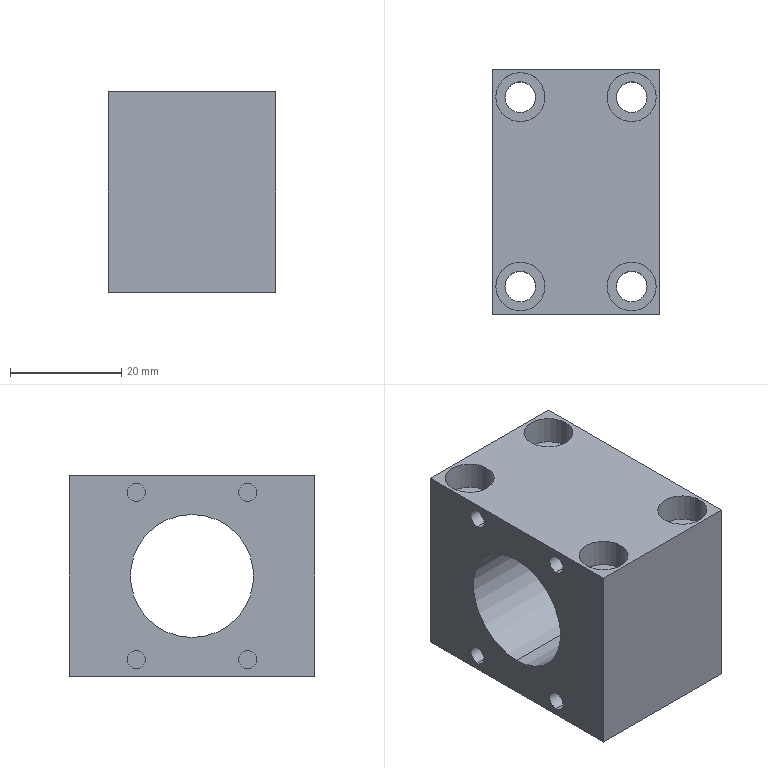Part | SolidWorks | features BaseBody 1 | 1 solid | 52 faces | box 30 x 44 x 36 mm | volume 31000 mm3 | cylinder 34 | plane 18 | commonest cylinder face diameters 3.3 x16 5.5 x8 8.8 x8 22.1 x2
STEP:
#1=CARTESIAN_POINT('',(-15.,0.,29.05));
#2=VERTEX_POINT('',#1);
#3=CARTESIAN_POINT('',(-15.,0.,6.95));
#4=VERTEX_POINT('',#3);
#5=CARTESIAN_POINT('',(-15.,0.,18.));
#6=DIRECTION('',(1.,0.,0.));
#7=DIRECTION('',(0.,0.,-1.));
#8=AXIS2_PLACEMENT_3D('',#5,#6,#7);
#9=CIRCLE('',#8,11.05);
#10=EDGE_CURVE('',#2,#4,#9,.T.);
#11=ORIENTED_EDGE('',*,*,#10,.F.);
#12=CARTESIAN_POINT('',(15.,0.,29.05));
#13=VERTEX_POINT('',#12);
#14=CARTESIAN_POINT('',(-16.,0.,29.05));
#15=DIRECTION('',(1.,0.,0.));
#16=VECTOR('',#15,1000.);
#17=LINE('',#14,#16);
#18=EDGE_CURVE('',#2,#13,#17,.T.);
#19=ORIENTED_EDGE('',*,*,#18,.T.);
#20=CARTESIAN_POINT('',(15.,0.,6.95));
#21=VERTEX_POINT('',#20);
#22=CARTESIAN_POINT('',(15.,0.,18.));
#23=DIRECTION('',(-1.,0.,0.));
#24=DIRECTION('',(0.,0.,-1.));
#25=AXIS2_PLACEMENT_3D('',#22,#23,#24);
#26=CIRCLE('',#25,11.05);
#27=EDGE_CURVE('',#21,#13,#26,.T.);
#28=ORIENTED_EDGE('',*,*,#27,.F.);
#29=CARTESIAN_POINT('',(-16.,0.,6.95));
#30=DIRECTION('',(1.,0.,0.));
#31=VECTOR('',#30,1000.);
#32=LINE('',#29,#31);
#33=EDGE_CURVE('',#4,#21,#32,.T.);
#34=ORIENTED_EDGE('',*,*,#33,.F.);
#35=EDGE_LOOP('',(#11,#19,#28,#34));
#36=FACE_OUTER_BOUND('',#35,.T.);
#37=CARTESIAN_POINT('',(-16.,0.,18.));
#38=DIRECTION('',(1.,0.,0.));
#39=DIRECTION('',(0.,0.,-1.));
#40=AXIS2_PLACEMENT_3D('',#37,#38,#39);
#41=CYLINDRICAL_SURFACE('',#40,11.05);
#42=ADVANCED_FACE('',(#36),#41,.F.);
#43=CARTESIAN_POINT('',(-2.8,-10.,31.35));
#44=VERTEX_POINT('',#43);
#45=CARTESIAN_POINT('',(-2.8,-10.,34.65));
#46=VERTEX_POINT('',#45);
#47=CARTESIAN_POINT('',(-2.8,-10.,33.));
#48=DIRECTION('',(-1.,0.,0.));
#49=DIRECTION('',(0.,0.,1.));
#50=AXIS2_PLACEMENT_3D('',#47,#48,#49);
#51=CIRCLE('',#50,1.65);
#52=EDGE_CURVE('',#44,#46,#51,.T.);
#53=ORIENTED_EDGE('',*,*,#52,.F.);
#54=CARTESIAN_POINT('',(-15.,-10.,31.35));
#55=VERTEX_POINT('',#54);
#56=CARTESIAN_POINT('',(-2.8,-10.,31.35));
#57=DIRECTION('',(-1.,0.,0.));
#58=VECTOR('',#57,1000.);
#59=LINE('',#56,#58);
#60=EDGE_CURVE('',#44,#55,#59,.T.);
#61=ORIENTED_EDGE('',*,*,#60,.T.);
#62=CARTESIAN_POINT('',(-15.,-10.,34.65));
#63=VERTEX_POINT('',#62);
#64=CARTESIAN_POINT('',(-15.,-10.,33.));
#65=DIRECTION('',(-1.,0.,0.));
#66=DIRECTION('',(0.,0.,1.));
#67=AXIS2_PLACEMENT_3D('',#64,#65,#66);
#68=CIRCLE('',#67,1.65);
#69=EDGE_CURVE('',#55,#63,#68,.T.);
#70=ORIENTED_EDGE('',*,*,#69,.T.);
#71=CARTESIAN_POINT('',(-2.8,-10.,34.65));
#72=DIRECTION('',(-1.,0.,0.));
#73=VECTOR('',#72,1000.);
#74=LINE('',#71,#73);
#75=EDGE_CURVE('',#46,#63,#74,.T.);
#76=ORIENTED_EDGE('',*,*,#75,.F.);
#77=EDGE_LOOP('',(#53,#61,#70,#76));
#78=FACE_OUTER_BOUND('',#77,.T.);
#79=CARTESIAN_POINT('',(-2.8,-10.,33.));
#80=DIRECTION('',(-1.,0.,0.));
#81=DIRECTION('',(0.,0.,1.));
#82=AXIS2_PLACEMENT_3D('',#79,#80,#81);
#83=CYLINDRICAL_SURFACE('',#82,1.65);
#84=ADVANCED_FACE('',(#78),#83,.F.);
#85=CARTESIAN_POINT('',(-2.8,-10.,1.35));
#86=VERTEX_POINT('',#85);
#87=CARTESIAN_POINT('',(-2.8,-10.,4.65));
#88=VERTEX_POINT('',#87);
#89=CARTESIAN_POINT('',(-2.8,-10.,3.));
#90=DIRECTION('',(-1.,0.,0.));
#91=DIRECTION('',(0.,0.,1.));
#92=AXIS2_PLACEMENT_3D('',#89,#90,#91);
#93=CIRCLE('',#92,1.65);
#94=EDGE_CURVE('',#86,#88,#93,.T.);
#95=ORIENTED_EDGE('',*,*,#94,.F.);
#96=CARTESIAN_POINT('',(-15.,-10.,1.35));
#97=VERTEX_POINT('',#96);
#98=CARTESIAN_POINT('',(-2.8,-10.,1.35));
#99=DIRECTION('',(-1.,0.,0.));
#100=VECTOR('',#99,1000.);
#101=LINE('',#98,#100);
#102=EDGE_CURVE('',#86,#97,#101,.T.);
#103=ORIENTED_EDGE('',*,*,#102,.T.);
#104=CARTESIAN_POINT('',(-15.,-10.,4.65));
#105=VERTEX_POINT('',#104);
#106=CARTESIAN_POINT('',(-15.,-10.,3.));
#107=DIRECTION('',(-1.,0.,0.));
#108=DIRECTION('',(0.,0.,1.));
#109=AXIS2_PLACEMENT_3D('',#106,#107,#108);
#110=CIRCLE('',#109,1.65);
#111=EDGE_CURVE('',#97,#105,#110,.T.);
#112=ORIENTED_EDGE('',*,*,#111,.T.);
#113=CARTESIAN_POINT('',(-2.8,-10.,4.65));
#114=DIRECTION('',(-1.,0.,0.));
#115=VECTOR('',#114,1000.);
#116=LINE('',#113,#115);
#117=EDGE_CURVE('',#88,#105,#116,.T.);
#118=ORIENTED_EDGE('',*,*,#117,.F.);
#119=EDGE_LOOP('',(#95,#103,#112,#118));
#120=FACE_OUTER_BOUND('',#119,.T.);
#121=CARTESIAN_POINT('',(-2.8,-10.,3.));
#122=DIRECTION('',(-1.,0.,0.));
#123=DIRECTION('',(0.,0.,1.));
#124=AXIS2_PLACEMENT_3D('',#121,#122,#123);
#125=CYLINDRICAL_SURFACE('',#124,1.65);
#126=ADVANCED_FACE('',(#120),#125,.F.);
#127=CARTESIAN_POINT('',(-2.8,10.,31.35));
#128=VERTEX_POINT('',#127);
#129=CARTESIAN_POINT('',(-2.8,10.,34.65));
#130=VERTEX_POINT('',#129);
#131=CARTESIAN_POINT('',(-2.8,10.,33.));
#132=DIRECTION('',(-1.,0.,0.));
#133=DIRECTION('',(0.,0.,1.));
#134=AXIS2_PLACEMENT_3D('',#131,#132,#133);
#135=CIRCLE('',#134,1.65);
#136=EDGE_CURVE('',#128,#130,#135,.T.);
#137=ORIENTED_EDGE('',*,*,#136,.F.);
#138=CARTESIAN_POINT('',(-15.,10.,31.35));
#139=VERTEX_POINT('',#138);
#140=CARTESIAN_POINT('',(-2.8,10.,31.35));
#141=DIRECTION('',(-1.,0.,0.));
#142=VECTOR('',#141,1000.);
#143=LINE('',#140,#142);
#144=EDGE_CURVE('',#128,#139,#143,.T.);
#145=ORIENTED_EDGE('',*,*,#144,.T.);
#146=CARTESIAN_POINT('',(-15.,10.,34.65));
#147=VERTEX_POINT('',#146);
#148=CARTESIAN_POINT('',(-15.,10.,33.));
#149=DIRECTION('',(-1.,0.,0.));
#150=DIRECTION('',(0.,0.,1.));
#151=AXIS2_PLACEMENT_3D('',#148,#149,#150);
#152=CIRCLE('',#151,1.65);
#153=EDGE_CURVE('',#139,#147,#152,.T.);
#154=ORIENTED_EDGE('',*,*,#153,.T.);
#155=CARTESIAN_POINT('',(-2.8,10.,34.65));
#156=DIRECTION('',(-1.,0.,0.));
#157=VECTOR('',#156,1000.);
#158=LINE('',#155,#157);
#159=EDGE_CURVE('',#130,#147,#158,.T.);
#160=ORIENTED_EDGE('',*,*,#159,.F.);
#161=EDGE_LOOP('',(#137,#145,#154,#160));
#162=FACE_OUTER_BOUND('',#161,.T.);
#163=CARTESIAN_POINT('',(-2.8,10.,33.));
#164=DIRECTION('',(-1.,0.,0.));
#165=DIRECTION('',(0.,0.,1.));
#166=AXIS2_PLACEMENT_3D('',#163,#164,#165);
#167=CYLINDRICAL_SURFACE('',#166,1.65);
#168=ADVANCED_FACE('',(#162),#167,.F.);
#169=CARTESIAN_POINT('',(-2.8,10.,1.35));
#170=VERTEX_POINT('',#169);
#171=CARTESIAN_POINT('',(-2.8,10.,4.65));
#172=VERTEX_POINT('',#171);
#173=CARTESIAN_POINT('',(-2.8,10.,3.));
#174=DIRECTION('',(-1.,0.,0.));
#175=DIRECTION('',(0.,0.,1.));
#176=AXIS2_PLACEMENT_3D('',#173,#174,#175);
#177=CIRCLE('',#176,1.65);
#178=EDGE_CURVE('',#170,#172,#177,.T.);
#179=ORIENTED_EDGE('',*,*,#178,.F.);
#180=CARTESIAN_POINT('',(-15.,10.,1.35));
#181=VERTEX_POINT('',#180);
#182=CARTESIAN_POINT('',(-2.8,10.,1.35));
#183=DIRECTION('',(-1.,0.,0.));
#184=VECTOR('',#183,1000.);
#185=LINE('',#182,#184);
#186=EDGE_CURVE('',#170,#181,#185,.T.);
#187=ORIENTED_EDGE('',*,*,#186,.T.);
#188=CARTESIAN_POINT('',(-15.,10.,4.65));
#189=VERTEX_POINT('',#188);
#190=CARTESIAN_POINT('',(-15.,10.,3.));
#191=DIRECTION('',(-1.,0.,0.));
#192=DIRECTION('',(0.,0.,1.));
#193=AXIS2_PLACEMENT_3D('',#190,#191,#192);
#194=CIRCLE('',#193,1.65);
#195=EDGE_CURVE('',#181,#189,#194,.T.);
#196=ORIENTED_EDGE('',*,*,#195,.T.);
#197=CARTESIAN_POINT('',(-2.8,10.,4.65));
#198=DIRECTION('',(-1.,0.,0.));
#199=VECTOR('',#198,1000.);
#200=LINE('',#197,#199);
#201=EDGE_CURVE('',#172,#189,#200,.T.);
#202=ORIENTED_EDGE('',*,*,#201,.F.);
#203=EDGE_LOOP('',(#179,#187,#196,#202));
#204=FACE_OUTER_BOUND('',#203,.T.);
#205=CARTESIAN_POINT('',(-2.8,10.,3.));
#206=DIRECTION('',(-1.,0.,0.));
#207=DIRECTION('',(0.,0.,1.));
#208=AXIS2_PLACEMENT_3D('',#205,#206,#207);
#209=CYLINDRICAL_SURFACE('',#208,1.65);
#210=ADVANCED_FACE('',(#204),#209,.F.);
#211=CARTESIAN_POINT('',(2.8,-10.,34.65));
#212=VERTEX_POINT('',#211);
#213=CARTESIAN_POINT('',(2.8,-10.,31.35));
#214=VERTEX_POINT('',#213);
#215=CARTESIAN_POINT('',(2.8,-10.,33.));
#216=DIRECTION('',(1.,0.,0.));
#217=DIRECTION('',(0.,0.,-1.));
#218=AXIS2_PLACEMENT_3D('',#215,#216,#217);
#219=CIRCLE('',#218,1.65);
#220=EDGE_CURVE('',#212,#214,#219,.T.);
#221=ORIENTED_EDGE('',*,*,#220,.F.);
#222=CARTESIAN_POINT('',(15.,-10.,34.65));
#223=VERTEX_POINT('',#222);
#224=CARTESIAN_POINT('',(2.8,-10.,34.65));
#225=DIRECTION('',(1.,0.,0.));
#226=VECTOR('',#225,1000.);
#227=LINE('',#224,#226);
#228=EDGE_CURVE('',#212,#223,#227,.T.);
#229=ORIENTED_EDGE('',*,*,#228,.T.);
#230=CARTESIAN_POINT('',(15.,-10.,31.35));
#231=VERTEX_POINT('',#230);
#232=CARTESIAN_POINT('',(15.,-10.,33.));
#233=DIRECTION('',(-1.,0.,0.));
#234=DIRECTION('',(0.,0.,-1.));
#235=AXIS2_PLACEMENT_3D('',#232,#233,#234);
#236=CIRCLE('',#235,1.65);
#237=EDGE_CURVE('',#231,#223,#236,.T.);
#238=ORIENTED_EDGE('',*,*,#237,.F.);
#239=CARTESIAN_POINT('',(2.8,-10.,31.35));
#240=DIRECTION('',(1.,0.,0.));
#241=VECTOR('',#240,1000.);
#242=LINE('',#239,#241);
#243=EDGE_CURVE('',#214,#231,#242,.T.);
#244=ORIENTED_EDGE('',*,*,#243,.F.);
#245=EDGE_LOOP('',(#221,#229,#238,#244));
#246=FACE_OUTER_BOUND('',#245,.T.);
#247=CARTESIAN_POINT('',(2.8,-10.,33.));
#248=DIRECTION('',(1.,0.,0.));
#249=DIRECTION('',(0.,0.,-1.));
#250=AXIS2_PLACEMENT_3D('',#247,#248,#249);
#251=CYLINDRICAL_SURFACE('',#250,1.65);
#252=ADVANCED_FACE('',(#246),#251,.F.);
#253=CARTESIAN_POINT('',(2.8,-10.,4.65));
#254=VERTEX_POINT('',#253);
#255=CARTESIAN_POINT('',(2.8,-10.,1.35));
#256=VERTEX_POINT('',#255);
#257=CARTESIAN_POINT('',(2.8,-10.,3.));
#258=DIRECTION('',(1.,0.,0.));
#259=DIRECTION('',(0.,0.,-1.));
#260=AXIS2_PLACEMENT_3D('',#257,#258,#259);
#261=CIRCLE('',#260,1.65);
#262=EDGE_CURVE('',#254,#256,#261,.T.);
#263=ORIENTED_EDGE('',*,*,#262,.F.);
#264=CARTESIAN_POINT('',(15.,-10.,4.65));
#265=VERTEX_POINT('',#264);
#266=CARTESIAN_POINT('',(2.8,-10.,4.65));
#267=DIRECTION('',(1.,0.,0.));
#268=VECTOR('',#267,1000.);
#269=LINE('',#266,#268);
#270=EDGE_CURVE('',#254,#265,#269,.T.);
#271=ORIENTED_EDGE('',*,*,#270,.T.);
#272=CARTESIAN_POINT('',(15.,-10.,1.35));
#273=VERTEX_POINT('',#272);
#274=CARTESIAN_POINT('',(15.,-10.,3.));
#275=DIRECTION('',(-1.,0.,0.));
#276=DIRECTION('',(0.,0.,-1.));
#277=AXIS2_PLACEMENT_3D('',#274,#275,#276);
#278=CIRCLE('',#277,1.65);
#279=EDGE_CURVE('',#273,#265,#278,.T.);
#280=ORIENTED_EDGE('',*,*,#279,.F.);
#281=CARTESIAN_POINT('',(2.8,-10.,1.35));
#282=DIRECTION('',(1.,0.,0.));
#283=VECTOR('',#282,1000.);
#284=LINE('',#281,#283);
#285=EDGE_CURVE('',#256,#273,#284,.T.);
#286=ORIENTED_EDGE('',*,*,#285,.F.);
#287=EDGE_LOOP('',(#263,#271,#280,#286));
#288=FACE_OUTER_BOUND('',#287,.T.);
#289=CARTESIAN_POINT('',(2.8,-10.,3.));
#290=DIRECTION('',(1.,0.,0.));
#291=DIRECTION('',(0.,0.,-1.));
#292=AXIS2_PLACEMENT_3D('',#289,#290,#291);
#293=CYLINDRICAL_SURFACE('',#292,1.65);
#294=ADVANCED_FACE('',(#288),#293,.F.);
#295=CARTESIAN_POINT('',(2.8,10.,34.65));
#296=VERTEX_POINT('',#295);
#297=CARTESIAN_POINT('',(2.8,10.,31.35));
#298=VERTEX_POINT('',#297);
#299=CARTESIAN_POINT('',(2.8,10.,33.));
#300=DIRECTION('',(1.,0.,0.));
#301=DIRECTION('',(0.,0.,-1.));
#302=AXIS2_PLACEMENT_3D('',#299,#300,#301);
#303=CIRCLE('',#302,1.65);
#304=EDGE_CURVE('',#296,#298,#303,.T.);
#305=ORIENTED_EDGE('',*,*,#304,.F.);
#306=CARTESIAN_POINT('',(15.,10.,34.65));
#307=VERTEX_POINT('',#306);
#308=CARTESIAN_POINT('',(2.8,10.,34.65));
#309=DIRECTION('',(1.,0.,0.));
#310=VECTOR('',#309,1000.);
#311=LINE('',#308,#310);
#312=EDGE_CURVE('',#296,#307,#311,.T.);
#313=ORIENTED_EDGE('',*,*,#312,.T.);
#314=CARTESIAN_POINT('',(15.,10.,31.35));
#315=VERTEX_POINT('',#314);
#316=CARTESIAN_POINT('',(15.,10.,33.));
#317=DIRECTION('',(-1.,0.,0.));
#318=DIRECTION('',(0.,0.,-1.));
#319=AXIS2_PLACEMENT_3D('',#316,#317,#318);
#320=CIRCLE('',#319,1.65);
#321=EDGE_CURVE('',#315,#307,#320,.T.);
#322=ORIENTED_EDGE('',*,*,#321,.F.);
#323=CARTESIAN_POINT('',(2.8,10.,31.35));
#324=DIRECTION('',(1.,0.,0.));
#325=VECTOR('',#324,1000.);
#326=LINE('',#323,#325);
#327=EDGE_CURVE('',#298,#315,#326,.T.);
#328=ORIENTED_EDGE('',*,*,#327,.F.);
#329=EDGE_LOOP('',(#305,#313,#322,#328));
#330=FACE_OUTER_BOUND('',#329,.T.);
#331=CARTESIAN_POINT('',(2.8,10.,33.));
#332=DIRECTION('',(1.,0.,0.));
#333=DIRECTION('',(0.,0.,-1.));
#334=AXIS2_PLACEMENT_3D('',#331,#332,#333);
#335=CYLINDRICAL_SURFACE('',#334,1.65);
#336=ADVANCED_FACE('',(#330),#335,.F.);
#337=CARTESIAN_POINT('',(2.8,10.,4.65));
#338=VERTEX_POINT('',#337);
#339=CARTESIAN_POINT('',(2.8,10.,1.35));
#340=VERTEX_POINT('',#339);
#341=CARTESIAN_POINT('',(2.8,10.,3.));
#342=DIRECTION('',(1.,0.,0.));
#343=DIRECTION('',(0.,0.,-1.));
#344=AXIS2_PLACEMENT_3D('',#341,#342,#343);
#345=CIRCLE('',#344,1.65);
#346=EDGE_CURVE('',#338,#340,#345,.T.);
#347=ORIENTED_EDGE('',*,*,#346,.F.);
#348=CARTESIAN_POINT('',(15.,10.,4.65));
#349=VERTEX_POINT('',#348);
#350=CARTESIAN_POINT('',(2.8,10.,4.65));
#351=DIRECTION('',(1.,0.,0.));
#352=VECTOR('',#351,1000.);
#353=LINE('',#350,#352);
#354=EDGE_CURVE('',#338,#349,#353,.T.);
#355=ORIENTED_EDGE('',*,*,#354,.T.);
#356=CARTESIAN_POINT('',(15.,10.,1.35));
#357=VERTEX_POINT('',#356);
#358=CARTESIAN_POINT('',(15.,10.,3.));
#359=DIRECTION('',(-1.,0.,0.));
#360=DIRECTION('',(0.,0.,-1.));
#361=AXIS2_PLACEMENT_3D('',#358,#359,#360);
#362=CIRCLE('',#361,1.65);
#363=EDGE_CURVE('',#357,#349,#362,.T.);
#364=ORIENTED_EDGE('',*,*,#363,.F.);
#365=CARTESIAN_POINT('',(2.8,10.,1.35));
#366=DIRECTION('',(1.,0.,0.));
#367=VECTOR('',#366,1000.);
#368=LINE('',#365,#367);
#369=EDGE_CURVE('',#340,#357,#368,.T.);
#370=ORIENTED_EDGE('',*,*,#369,.F.);
#371=EDGE_LOOP('',(#347,#355,#364,#370));
#372=FACE_OUTER_BOUND('',#371,.T.);
#373=CARTESIAN_POINT('',(2.8,10.,3.));
#374=DIRECTION('',(1.,0.,0.));
#375=DIRECTION('',(0.,0.,-1.));
#376=AXIS2_PLACEMENT_3D('',#373,#374,#375);
#377=CYLINDRICAL_SURFACE('',#376,1.65);
#378=ADVANCED_FACE('',(#372),#377,.F.);
#379=CARTESIAN_POINT('',(5.6,17.,30.9));
#380=VERTEX_POINT('',#379);
#381=CARTESIAN_POINT('',(14.4,17.,30.9));
#382=VERTEX_POINT('',#381);
#383=CARTESIAN_POINT('',(10.,17.,30.9));
#384=DIRECTION('',(0.,0.,1.));
#385=DIRECTION('',(1.,0.,0.));
#386=AXIS2_PLACEMENT_3D('',#383,#384,#385);
#387=CIRCLE('',#386,4.4);
#388=EDGE_CURVE('',#380,#382,#387,.T.);
#389=ORIENTED_EDGE('',*,*,#388,.F.);
#390=CARTESIAN_POINT('',(5.6,17.,36.));
#391=VERTEX_POINT('',#390);
#392=CARTESIAN_POINT('',(5.6,17.,30.9));
#393=DIRECTION('',(0.,0.,1.));
#394=VECTOR('',#393,1000.);
#395=LINE('',#392,#394);
#396=EDGE_CURVE('',#380,#391,#395,.T.);
#397=ORIENTED_EDGE('',*,*,#396,.T.);
#398=CARTESIAN_POINT('',(14.4,17.,36.));
#399=VERTEX_POINT('',#398);
#400=CARTESIAN_POINT('',(10.,17.,36.));
#401=DIRECTION('',(0.,0.,-1.));
#402=DIRECTION('',(1.,0.,0.));
#403=AXIS2_PLACEMENT_3D('',#400,#401,#402);
#404=CIRCLE('',#403,4.4);
#405=EDGE_CURVE('',#399,#391,#404,.T.);
#406=ORIENTED_EDGE('',*,*,#405,.F.);
#407=CARTESIAN_POINT('',(14.4,17.,30.9));
#408=DIRECTION('',(0.,0.,1.));
#409=VECTOR('',#408,1000.);
#410=LINE('',#407,#409);
#411=EDGE_CURVE('',#382,#399,#410,.T.);
#412=ORIENTED_EDGE('',*,*,#411,.F.);
#413=EDGE_LOOP('',(#389,#397,#406,#412));
#414=FACE_OUTER_BOUND('',#413,.T.);
#415=CARTESIAN_POINT('',(10.,17.,30.9));
#416=DIRECTION('',(0.,0.,1.));
#417=DIRECTION('',(1.,0.,0.));
#418=AXIS2_PLACEMENT_3D('',#415,#416,#417);
#419=CYLINDRICAL_SURFACE('',#418,4.4);
#420=ADVANCED_FACE('',(#414),#419,.F.);
#421=CARTESIAN_POINT('',(-14.4,17.,30.9));
#422=VERTEX_POINT('',#421);
#423=CARTESIAN_POINT('',(-5.6,17.,30.9));
#424=VERTEX_POINT('',#423);
#425=CARTESIAN_POINT('',(-10.,17.,30.9));
#426=DIRECTION('',(0.,0.,1.));
#427=DIRECTION('',(1.,0.,0.));
#428=AXIS2_PLACEMENT_3D('',#425,#426,#427);
#429=CIRCLE('',#428,4.4);
#430=EDGE_CURVE('',#422,#424,#429,.T.);
#431=ORIENTED_EDGE('',*,*,#430,.F.);
#432=CARTESIAN_POINT('',(-14.4,17.,36.));
#433=VERTEX_POINT('',#432);
#434=CARTESIAN_POINT('',(-14.4,17.,30.9));
#435=DIRECTION('',(0.,0.,1.));
#436=VECTOR('',#435,1000.);
#437=LINE('',#434,#436);
#438=EDGE_CURVE('',#422,#433,#437,.T.);
#439=ORIENTED_EDGE('',*,*,#438,.T.);
#440=CARTESIAN_POINT('',(-5.6,17.,36.));
#441=VERTEX_POINT('',#440);
#442=CARTESIAN_POINT('',(-10.,17.,36.));
#443=DIRECTION('',(0.,0.,-1.));
#444=DIRECTION('',(1.,0.,0.));
#445=AXIS2_PLACEMENT_3D('',#442,#443,#444);
#446=CIRCLE('',#445,4.4);
#447=EDGE_CURVE('',#441,#433,#446,.T.);
#448=ORIENTED_EDGE('',*,*,#447,.F.);
#449=CARTESIAN_POINT('',(-5.6,17.,30.9));
#450=DIRECTION('',(0.,0.,1.));
#451=VECTOR('',#450,1000.);
#452=LINE('',#449,#451);
#453=EDGE_CURVE('',#424,#441,#452,.T.);
#454=ORIENTED_EDGE('',*,*,#453,.F.);
#455=EDGE_LOOP('',(#431,#439,#448,#454));
#456=FACE_OUTER_BOUND('',#455,.T.);
#457=CARTESIAN_POINT('',(-10.,17.,30.9));
#458=DIRECTION('',(0.,0.,1.));
#459=DIRECTION('',(1.,0.,0.));
#460=AXIS2_PLACEMENT_3D('',#457,#458,#459);
#461=CYLINDRICAL_SURFACE('',#460,4.4);
#462=ADVANCED_FACE('',(#456),#461,.F.);
#463=CARTESIAN_POINT('',(5.6,-17.,30.9));
#464=VERTEX_POINT('',#463);
#465=CARTESIAN_POINT('',(14.4,-17.,30.9));
#466=VERTEX_POINT('',#465);
#467=CARTESIAN_POINT('',(10.,-17.,30.9));
#468=DIRECTION('',(0.,0.,1.));
#469=DIRECTION('',(1.,0.,0.));
#470=AXIS2_PLACEMENT_3D('',#467,#468,#469);
#471=CIRCLE('',#470,4.4);
#472=EDGE_CURVE('',#464,#466,#471,.T.);
#473=ORIENTED_EDGE('',*,*,#472,.F.);
#474=CARTESIAN_POINT('',(5.6,-17.,36.));
#475=VERTEX_POINT('',#474);
#476=CARTESIAN_POINT('',(5.6,-17.,30.9));
#477=DIRECTION('',(0.,0.,1.));
#478=VECTOR('',#477,1000.);
#479=LINE('',#476,#478);
#480=EDGE_CURVE('',#464,#475,#479,.T.);
#481=ORIENTED_EDGE('',*,*,#480,.T.);
#482=CARTESIAN_POINT('',(14.4,-17.,36.));
#483=VERTEX_POINT('',#482);
#484=CARTESIAN_POINT('',(10.,-17.,36.));
#485=DIRECTION('',(0.,0.,-1.));
#486=DIRECTION('',(1.,0.,0.));
#487=AXIS2_PLACEMENT_3D('',#484,#485,#486);
#488=CIRCLE('',#487,4.4);
#489=EDGE_CURVE('',#483,#475,#488,.T.);
#490=ORIENTED_EDGE('',*,*,#489,.F.);
#491=CARTESIAN_POINT('',(14.4,-17.,30.9));
#492=DIRECTION('',(0.,0.,1.));
#493=VECTOR('',#492,1000.);
#494=LINE('',#491,#493);
#495=EDGE_CURVE('',#466,#483,#494,.T.);
#496=ORIENTED_EDGE('',*,*,#495,.F.);
#497=EDGE_LOOP('',(#473,#481,#490,#496));
#498=FACE_OUTER_BOUND('',#497,.T.);
#499=CARTESIAN_POINT('',(10.,-17.,30.9));
#500=DIRECTION('',(0.,0.,1.));
#501=DIRECTION('',(1.,0.,0.));
#502=AXIS2_PLACEMENT_3D('',#499,#500,#501);
#503=CYLINDRICAL_SURFACE('',#502,4.4);
#504=ADVANCED_FACE('',(#498),#503,.F.);
#505=CARTESIAN_POINT('',(-14.4,-17.,30.9));
#506=VERTEX_POINT('',#505);
#507=CARTESIAN_POINT('',(-5.6,-17.,30.9));
#508=VERTEX_POINT('',#507);
#509=CARTESIAN_POINT('',(-10.,-17.,30.9));
#510=DIRECTION('',(0.,0.,1.));
#511=DIRECTION('',(1.,0.,0.));
#512=AXIS2_PLACEMENT_3D('',#509,#510,#511);
#513=CIRCLE('',#512,4.4);
#514=EDGE_CURVE('',#506,#508,#513,.T.);
#515=ORIENTED_EDGE('',*,*,#514,.F.);
#516=CARTESIAN_POINT('',(-14.4,-17.,36.));
#517=VERTEX_POINT('',#516);
#518=CARTESIAN_POINT('',(-14.4,-17.,30.9));
#519=DIRECTION('',(0.,0.,1.));
#520=VECTOR('',#519,1000.);
#521=LINE('',#518,#520);
#522=EDGE_CURVE('',#506,#517,#521,.T.);
#523=ORIENTED_EDGE('',*,*,#522,.T.);
#524=CARTESIAN_POINT('',(-5.6,-17.,36.));
#525=VERTEX_POINT('',#524);
#526=CARTESIAN_POINT('',(-10.,-17.,36.));
#527=DIRECTION('',(0.,0.,-1.));
#528=DIRECTION('',(1.,0.,0.));
#529=AXIS2_PLACEMENT_3D('',#526,#527,#528);
#530=CIRCLE('',#529,4.4);
#531=EDGE_CURVE('',#525,#517,#530,.T.);
#532=ORIENTED_EDGE('',*,*,#531,.F.);
#533=CARTESIAN_POINT('',(-5.6,-17.,30.9));
#534=DIRECTION('',(0.,0.,1.));
#535=VECTOR('',#534,1000.);
#536=LINE('',#533,#535);
#537=EDGE_CURVE('',#508,#525,#536,.T.);
#538=ORIENTED_EDGE('',*,*,#537,.F.);
#539=EDGE_LOOP('',(#515,#523,#532,#538));
#540=FACE_OUTER_BOUND('',#539,.T.);
#541=CARTESIAN_POINT('',(-10.,-17.,30.9));
#542=DIRECTION('',(0.,0.,1.));
#543=DIRECTION('',(1.,0.,0.));
#544=AXIS2_PLACEMENT_3D('',#541,#542,#543);
#545=CYLINDRICAL_SURFACE('',#544,4.4);
#546=ADVANCED_FACE('',(#540),#545,.F.);
#547=CARTESIAN_POINT('',(12.75,17.,0.));
#548=VERTEX_POINT('',#547);
#549=CARTESIAN_POINT('',(7.25,17.,0.));
#550=VERTEX_POINT('',#549);
#551=CARTESIAN_POINT('',(10.,17.,0.));
#552=DIRECTION('',(0.,0.,-1.));
#553=DIRECTION('',(1.,0.,0.));
#554=AXIS2_PLACEMENT_3D('',#551,#552,#553);
#555=CIRCLE('',#554,2.75);
#556=EDGE_CURVE('',#548,#550,#555,.T.);
#557=ORIENTED_EDGE('',*,*,#556,.T.);
#558=CARTESIAN_POINT('',(7.25,17.,30.9));
#559=VERTEX_POINT('',#558);
#560=CARTESIAN_POINT('',(7.25,17.,-1.));
#561=DIRECTION('',(0.,0.,1.));
#562=VECTOR('',#561,1000.);
#563=LINE('',#560,#562);
#564=EDGE_CURVE('',#550,#559,#563,.T.);
#565=ORIENTED_EDGE('',*,*,#564,.T.);
#566=CARTESIAN_POINT('',(12.75,17.,30.9));
#567=VERTEX_POINT('',#566);
#568=CARTESIAN_POINT('',(10.,17.,30.9));
#569=DIRECTION('',(0.,0.,-1.));
#570=DIRECTION('',(1.,0.,0.));
#571=AXIS2_PLACEMENT_3D('',#568,#569,#570);
#572=CIRCLE('',#571,2.75);
#573=EDGE_CURVE('',#567,#559,#572,.T.);
#574=ORIENTED_EDGE('',*,*,#573,.F.);
#575=CARTESIAN_POINT('',(12.75,17.,-1.));
#576=DIRECTION('',(0.,0.,1.));
#577=VECTOR('',#576,1000.);
#578=LINE('',#575,#577);
#579=EDGE_CURVE('',#548,#567,#578,.T.);
#580=ORIENTED_EDGE('',*,*,#579,.F.);
#581=EDGE_LOOP('',(#557,#565,#574,#580));
#582=FACE_OUTER_BOUND('',#581,.T.);
#583=CARTESIAN_POINT('',(10.,17.,-1.));
#584=DIRECTION('',(0.,0.,1.));
#585=DIRECTION('',(1.,0.,0.));
#586=AXIS2_PLACEMENT_3D('',#583,#584,#585);
#587=CYLINDRICAL_SURFACE('',#586,2.75);
#588=ADVANCED_FACE('',(#582),#587,.F.);
#589=CARTESIAN_POINT('',(-7.25,17.,0.));
#590=VERTEX_POINT('',#589);
#591=CARTESIAN_POINT('',(-12.75,17.,0.));
#592=VERTEX_POINT('',#591);
#593=CARTESIAN_POINT('',(-10.,17.,0.));
#594=DIRECTION('',(0.,0.,-1.));
#595=DIRECTION('',(1.,0.,0.));
#596=AXIS2_PLACEMENT_3D('',#593,#594,#595);
#597=CIRCLE('',#596,2.75);
#598=EDGE_CURVE('',#590,#592,#597,.T.);
#599=ORIENTED_EDGE('',*,*,#598,.T.);
#600=CARTESIAN_POINT('',(-12.75,17.,30.9));
#601=VERTEX_POINT('',#600);
#602=CARTESIAN_POINT('',(-12.75,17.,-1.));
#603=DIRECTION('',(0.,0.,1.));
#604=VECTOR('',#603,1000.);
#605=LINE('',#602,#604);
#606=EDGE_CURVE('',#592,#601,#605,.T.);
#607=ORIENTED_EDGE('',*,*,#606,.T.);
#608=CARTESIAN_POINT('',(-7.25,17.,30.9));
#609=VERTEX_POINT('',#608);
#610=CARTESIAN_POINT('',(-10.,17.,30.9));
#611=DIRECTION('',(0.,0.,-1.));
#612=DIRECTION('',(1.,0.,0.));
#613=AXIS2_PLACEMENT_3D('',#610,#611,#612);
#614=CIRCLE('',#613,2.75);
#615=EDGE_CURVE('',#609,#601,#614,.T.);
#616=ORIENTED_EDGE('',*,*,#615,.F.);
#617=CARTESIAN_POINT('',(-7.25,17.,-1.));
#618=DIRECTION('',(0.,0.,1.));
#619=VECTOR('',#618,1000.);
#620=LINE('',#617,#619);
#621=EDGE_CURVE('',#590,#609,#620,.T.);
#622=ORIENTED_EDGE('',*,*,#621,.F.);
#623=EDGE_LOOP('',(#599,#607,#616,#622));
#624=FACE_OUTER_BOUND('',#623,.T.);
#625=CARTESIAN_POINT('',(-10.,17.,-1.));
#626=DIRECTION('',(0.,0.,1.));
#627=DIRECTION('',(1.,0.,0.));
#628=AXIS2_PLACEMENT_3D('',#625,#626,#627);
#629=CYLINDRICAL_SURFACE('',#628,2.75);
#630=ADVANCED_FACE('',(#624),#629,.F.);
#631=CARTESIAN_POINT('',(12.75,-17.,0.));
#632=VERTEX_POINT('',#631);
#633=CARTESIAN_POINT('',(7.25,-17.,0.));
#634=VERTEX_POINT('',#633);
#635=CARTESIAN_POINT('',(10.,-17.,0.));
#636=DIRECTION('',(0.,0.,-1.));
#637=DIRECTION('',(1.,0.,0.));
#638=AXIS2_PLACEMENT_3D('',#635,#636,#637);
#639=CIRCLE('',#638,2.75);
#640=EDGE_CURVE('',#632,#634,#639,.T.);
#641=ORIENTED_EDGE('',*,*,#640,.T.);
#642=CARTESIAN_POINT('',(7.25,-17.,30.9));
#643=VERTEX_POINT('',#642);
#644=CARTESIAN_POINT('',(7.25,-17.,-1.));
#645=DIRECTION('',(0.,0.,1.));
#646=VECTOR('',#645,1000.);
#647=LINE('',#644,#646);
#648=EDGE_CURVE('',#634,#643,#647,.T.);
#649=ORIENTED_EDGE('',*,*,#648,.T.);
#650=CARTESIAN_POINT('',(12.75,-17.,30.9));
#651=VERTEX_POINT('',#650);
#652=CARTESIAN_POINT('',(10.,-17.,30.9));
#653=DIRECTION('',(0.,0.,-1.));
#654=DIRECTION('',(1.,0.,0.));
#655=AXIS2_PLACEMENT_3D('',#652,#653,#654);
#656=CIRCLE('',#655,2.75);
#657=EDGE_CURVE('',#651,#643,#656,.T.);
#658=ORIENTED_EDGE('',*,*,#657,.F.);
#659=CARTESIAN_POINT('',(12.75,-17.,-1.));
#660=DIRECTION('',(0.,0.,1.));
#661=VECTOR('',#660,1000.);
#662=LINE('',#659,#661);
#663=EDGE_CURVE('',#632,#651,#662,.T.);
#664=ORIENTED_EDGE('',*,*,#663,.F.);
#665=EDGE_LOOP('',(#641,#649,#658,#664));
#666=FACE_OUTER_BOUND('',#665,.T.);
#667=CARTESIAN_POINT('',(10.,-17.,-1.));
#668=DIRECTION('',(0.,0.,1.));
#669=DIRECTION('',(1.,0.,0.));
#670=AXIS2_PLACEMENT_3D('',#667,#668,#669);
#671=CYLINDRICAL_SURFACE('',#670,2.75);
#672=ADVANCED_FACE('',(#666),#671,.F.);
#673=CARTESIAN_POINT('',(-7.25,-17.,0.));
#674=VERTEX_POINT('',#673);
#675=CARTESIAN_POINT('',(-12.75,-17.,0.));
#676=VERTEX_POINT('',#675);
#677=CARTESIAN_POINT('',(-10.,-17.,0.));
#678=DIRECTION('',(0.,0.,-1.));
#679=DIRECTION('',(1.,0.,0.));
#680=AXIS2_PLACEMENT_3D('',#677,#678,#679);
#681=CIRCLE('',#680,2.75);
#682=EDGE_CURVE('',#674,#676,#681,.T.);
#683=ORIENTED_EDGE('',*,*,#682,.T.);
#684=CARTESIAN_POINT('',(-12.75,-17.,30.9));
#685=VERTEX_POINT('',#684);
#686=CARTESIAN_POINT('',(-12.75,-17.,-1.));
#687=DIRECTION('',(0.,0.,1.));
#688=VECTOR('',#687,1000.);
#689=LINE('',#686,#688);
#690=EDGE_CURVE('',#676,#685,#689,.T.);
#691=ORIENTED_EDGE('',*,*,#690,.T.);
#692=CARTESIAN_POINT('',(-7.25,-17.,30.9));
#693=VERTEX_POINT('',#692);
#694=CARTESIAN_POINT('',(-10.,-17.,30.9));
#695=DIRECTION('',(0.,0.,-1.));
#696=DIRECTION('',(1.,0.,0.));
#697=AXIS2_PLACEMENT_3D('',#694,#695,#696);
#698=CIRCLE('',#697,2.75);
#699=EDGE_CURVE('',#693,#685,#698,.T.);
#700=ORIENTED_EDGE('',*,*,#699,.F.);
#701=CARTESIAN_POINT('',(-7.25,-17.,-1.));
#702=DIRECTION('',(0.,0.,1.));
#703=VECTOR('',#702,1000.);
#704=LINE('',#701,#703);
#705=EDGE_CURVE('',#674,#693,#704,.T.);
#706=ORIENTED_EDGE('',*,*,#705,.F.);
#707=EDGE_LOOP('',(#683,#691,#700,#706));
#708=FACE_OUTER_BOUND('',#707,.T.);
#709=CARTESIAN_POINT('',(-10.,-17.,-1.));
#710=DIRECTION('',(0.,0.,1.));
#711=DIRECTION('',(1.,0.,0.));
#712=AXIS2_PLACEMENT_3D('',#709,#710,#711);
#713=CYLINDRICAL_SURFACE('',#712,2.75);
#714=ADVANCED_FACE('',(#708),#713,.F.);
#715=ORIENTED_EDGE('',*,*,#18,.F.);
#716=CARTESIAN_POINT('',(-15.,0.,18.));
#717=DIRECTION('',(1.,0.,0.));
#718=DIRECTION('',(0.,0.,-1.));
#719=AXIS2_PLACEMENT_3D('',#716,#717,#718);
#720=CIRCLE('',#719,11.05);
#721=EDGE_CURVE('',#4,#2,#720,.T.);
#722=ORIENTED_EDGE('',*,*,#721,.F.);
#723=ORIENTED_EDGE('',*,*,#33,.T.);
#724=CARTESIAN_POINT('',(15.,0.,18.));
#725=DIRECTION('',(-1.,0.,0.));
#726=DIRECTION('',(0.,0.,-1.));
#727=AXIS2_PLACEMENT_3D('',#724,#725,#726);
#728=CIRCLE('',#727,11.05);
#729=EDGE_CURVE('',#13,#21,#728,.T.);
#730=ORIENTED_EDGE('',*,*,#729,.F.);
#731=EDGE_LOOP('',(#715,#722,#723,#730));
#732=FACE_OUTER_BOUND('',#731,.T.);
#733=CARTESIAN_POINT('',(-16.,0.,18.));
#734=DIRECTION('',(1.,0.,0.));
#735=DIRECTION('',(0.,0.,-1.));
#736=AXIS2_PLACEMENT_3D('',#733,#734,#735);
#737=CYLINDRICAL_SURFACE('',#736,11.05);
#738=ADVANCED_FACE('',(#732),#737,.F.);
#739=CARTESIAN_POINT('',(-15.,-10.,33.));
#740=DIRECTION('',(-1.,0.,0.));
#741=DIRECTION('',(0.,0.,1.));
#742=AXIS2_PLACEMENT_3D('',#739,#740,#741);
#743=CIRCLE('',#742,1.65);
#744=EDGE_CURVE('',#63,#55,#743,.T.);
#745=ORIENTED_EDGE('',*,*,#744,.F.);
#746=ORIENTED_EDGE('',*,*,#69,.F.);
#747=EDGE_LOOP('',(#745,#746));
#748=FACE_BOUND('',#747,.T.);
#749=ORIENTED_EDGE('',*,*,#721,.T.);
#750=ORIENTED_EDGE('',*,*,#10,.T.);
#751=EDGE_LOOP('',(#749,#750));
#752=FACE_BOUND('',#751,.T.);
#753=CARTESIAN_POINT('',(-15.,-10.,3.));
#754=DIRECTION('',(-1.,0.,0.));
#755=DIRECTION('',(0.,0.,1.));
#756=AXIS2_PLACEMENT_3D('',#753,#754,#755);
#757=CIRCLE('',#756,1.65);
#758=EDGE_CURVE('',#105,#97,#757,.T.);
#759=ORIENTED_EDGE('',*,*,#758,.F.);
#760=ORIENTED_EDGE('',*,*,#111,.F.);
#761=EDGE_LOOP('',(#759,#760));
#762=FACE_BOUND('',#761,.T.);
#763=CARTESIAN_POINT('',(-15.,10.,33.));
#764=DIRECTION('',(-1.,0.,0.));
#765=DIRECTION('',(0.,0.,1.));
#766=AXIS2_PLACEMENT_3D('',#763,#764,#765);
#767=CIRCLE('',#766,1.65);
#768=EDGE_CURVE('',#147,#139,#767,.T.);
#769=ORIENTED_EDGE('',*,*,#768,.F.);
#770=ORIENTED_EDGE('',*,*,#153,.F.);
#771=EDGE_LOOP('',(#769,#770));
#772=FACE_BOUND('',#771,.T.);
#773=CARTESIAN_POINT('',(-15.,10.,3.));
#774=DIRECTION('',(-1.,0.,0.));
#775=DIRECTION('',(0.,0.,1.));
#776=AXIS2_PLACEMENT_3D('',#773,#774,#775);
#777=CIRCLE('',#776,1.65);
#778=EDGE_CURVE('',#189,#181,#777,.T.);
#779=ORIENTED_EDGE('',*,*,#778,.F.);
#780=ORIENTED_EDGE('',*,*,#195,.F.);
#781=EDGE_LOOP('',(#779,#780));
#782=FACE_BOUND('',#781,.T.);
#783=CARTESIAN_POINT('',(-15.,22.,0.));
#784=VERTEX_POINT('',#783);
#785=CARTESIAN_POINT('',(-15.,22.,36.));
#786=VERTEX_POINT('',#785);
#787=CARTESIAN_POINT('',(-15.,22.,0.));
#788=DIRECTION('',(0.,0.,1.));
#789=VECTOR('',#788,1000.);
#790=LINE('',#787,#789);
#791=EDGE_CURVE('',#784,#786,#790,.T.);
#792=ORIENTED_EDGE('',*,*,#791,.F.);
#793=CARTESIAN_POINT('',(-15.,-22.,0.));
#794=VERTEX_POINT('',#793);
#795=CARTESIAN_POINT('',(-15.,-22.,0.));
#796=DIRECTION('',(0.,1.,0.));
#797=VECTOR('',#796,1000.);
#798=LINE('',#795,#797);
#799=EDGE_CURVE('',#794,#784,#798,.T.);
#800=ORIENTED_EDGE('',*,*,#799,.F.);
#801=CARTESIAN_POINT('',(-15.,-22.,36.));
#802=VERTEX_POINT('',#801);
#803=CARTESIAN_POINT('',(-15.,-22.,0.));
#804=DIRECTION('',(0.,0.,-1.));
#805=VECTOR('',#804,1000.);
#806=LINE('',#803,#805);
#807=EDGE_CURVE('',#802,#794,#806,.T.);
#808=ORIENTED_EDGE('',*,*,#807,.F.);
#809=CARTESIAN_POINT('',(-15.,-22.,36.));
#810=DIRECTION('',(0.,-1.,0.));
#811=VECTOR('',#810,1000.);
#812=LINE('',#809,#811);
#813=EDGE_CURVE('',#786,#802,#812,.T.);
#814=ORIENTED_EDGE('',*,*,#813,.F.);
#815=EDGE_LOOP('',(#792,#800,#808,#814));
#816=FACE_OUTER_BOUND('',#815,.T.);
#817=CARTESIAN_POINT('',(-15.,-22.,0.));
#818=DIRECTION('',(1.,0.,0.));
#819=DIRECTION('',(0.,0.,-1.));
#820=AXIS2_PLACEMENT_3D('',#817,#818,#819);
#821=PLANE('',#820);
#822=ADVANCED_FACE('',(#748,#752,#762,#772,#782,#816),#821,.F.);
#823=ORIENTED_EDGE('',*,*,#237,.T.);
#824=CARTESIAN_POINT('',(15.,-10.,33.));
#825=DIRECTION('',(-1.,0.,0.));
#826=DIRECTION('',(0.,0.,-1.));
#827=AXIS2_PLACEMENT_3D('',#824,#825,#826);
#828=CIRCLE('',#827,1.65);
#829=EDGE_CURVE('',#223,#231,#828,.T.);
#830=ORIENTED_EDGE('',*,*,#829,.T.);
#831=EDGE_LOOP('',(#823,#830));
#832=FACE_BOUND('',#831,.T.);
#833=ORIENTED_EDGE('',*,*,#27,.T.);
#834=ORIENTED_EDGE('',*,*,#729,.T.);
#835=EDGE_LOOP('',(#833,#834));
#836=FACE_BOUND('',#835,.T.);
#837=ORIENTED_EDGE('',*,*,#279,.T.);
#838=CARTESIAN_POINT('',(15.,-10.,3.));
#839=DIRECTION('',(-1.,0.,0.));
#840=DIRECTION('',(0.,0.,-1.));
#841=AXIS2_PLACEMENT_3D('',#838,#839,#840);
#842=CIRCLE('',#841,1.65);
#843=EDGE_CURVE('',#265,#273,#842,.T.);
#844=ORIENTED_EDGE('',*,*,#843,.T.);
#845=EDGE_LOOP('',(#837,#844));
#846=FACE_BOUND('',#845,.T.);
#847=ORIENTED_EDGE('',*,*,#321,.T.);
#848=CARTESIAN_POINT('',(15.,10.,33.));
#849=DIRECTION('',(-1.,0.,0.));
#850=DIRECTION('',(0.,0.,-1.));
#851=AXIS2_PLACEMENT_3D('',#848,#849,#850);
#852=CIRCLE('',#851,1.65);
#853=EDGE_CURVE('',#307,#315,#852,.T.);
#854=ORIENTED_EDGE('',*,*,#853,.T.);
#855=EDGE_LOOP('',(#847,#854));
#856=FACE_BOUND('',#855,.T.);
#857=ORIENTED_EDGE('',*,*,#363,.T.);
#858=CARTESIAN_POINT('',(15.,10.,3.));
#859=DIRECTION('',(-1.,0.,0.));
#860=DIRECTION('',(0.,0.,-1.));
#861=AXIS2_PLACEMENT_3D('',#858,#859,#860);
#862=CIRCLE('',#861,1.65);
#863=EDGE_CURVE('',#349,#357,#862,.T.);
#864=ORIENTED_EDGE('',*,*,#863,.T.);
#865=EDGE_LOOP('',(#857,#864));
#866=FACE_BOUND('',#865,.T.);
#867=CARTESIAN_POINT('',(15.,22.,0.));
#868=VERTEX_POINT('',#867);
#869=CARTESIAN_POINT('',(15.,22.,36.));
#870=VERTEX_POINT('',#869);
#871=CARTESIAN_POINT('',(15.,22.,0.));
#872=DIRECTION('',(0.,0.,1.));
#873=VECTOR('',#872,1000.);
#874=LINE('',#871,#873);
#875=EDGE_CURVE('',#868,#870,#874,.T.);
#876=ORIENTED_EDGE('',*,*,#875,.T.);
#877=CARTESIAN_POINT('',(15.,-22.,36.));
#878=VERTEX_POINT('',#877);
#879=CARTESIAN_POINT('',(15.,-22.,36.));
#880=DIRECTION('',(0.,-1.,0.));
#881=VECTOR('',#880,1000.);
#882=LINE('',#879,#881);
#883=EDGE_CURVE('',#870,#878,#882,.T.);
#884=ORIENTED_EDGE('',*,*,#883,.T.);
#885=CARTESIAN_POINT('',(15.,-22.,0.));
#886=VERTEX_POINT('',#885);
#887=CARTESIAN_POINT('',(15.,-22.,0.));
#888=DIRECTION('',(0.,0.,-1.));
#889=VECTOR('',#888,1000.);
#890=LINE('',#887,#889);
#891=EDGE_CURVE('',#878,#886,#890,.T.);
#892=ORIENTED_EDGE('',*,*,#891,.T.);
#893=CARTESIAN_POINT('',(15.,-22.,0.));
#894=DIRECTION('',(0.,1.,0.));
#895=VECTOR('',#894,1000.);
#896=LINE('',#893,#895);
#897=EDGE_CURVE('',#886,#868,#896,.T.);
#898=ORIENTED_EDGE('',*,*,#897,.T.);
#899=EDGE_LOOP('',(#876,#884,#892,#898));
#900=FACE_OUTER_BOUND('',#899,.T.);
#901=CARTESIAN_POINT('',(15.,-22.,0.));
#902=DIRECTION('',(1.,0.,0.));
#903=DIRECTION('',(0.,0.,-1.));
#904=AXIS2_PLACEMENT_3D('',#901,#902,#903);
#905=PLANE('',#904);
#906=ADVANCED_FACE('',(#832,#836,#846,#856,#866,#900),#905,.T.);
#907=ORIENTED_EDGE('',*,*,#60,.F.);
#908=CARTESIAN_POINT('',(-2.8,-10.,33.));
#909=DIRECTION('',(-1.,0.,0.));
#910=DIRECTION('',(0.,0.,1.));
#911=AXIS2_PLACEMENT_3D('',#908,#909,#910);
#912=CIRCLE('',#911,1.65);
#913=EDGE_CURVE('',#46,#44,#912,.T.);
#914=ORIENTED_EDGE('',*,*,#913,.F.);
#915=ORIENTED_EDGE('',*,*,#75,.T.);
#916=ORIENTED_EDGE('',*,*,#744,.T.);
#917=EDGE_LOOP('',(#907,#914,#915,#916));
#918=FACE_OUTER_BOUND('',#917,.T.);
#919=CARTESIAN_POINT('',(-2.8,-10.,33.));
#920=DIRECTION('',(-1.,0.,0.));
#921=DIRECTION('',(0.,0.,1.));
#922=AXIS2_PLACEMENT_3D('',#919,#920,#921);
#923=CYLINDRICAL_SURFACE('',#922,1.65);
#924=ADVANCED_FACE('',(#918),#923,.F.);
#925=ORIENTED_EDGE('',*,*,#102,.F.);
#926=CARTESIAN_POINT('',(-2.8,-10.,3.));
#927=DIRECTION('',(-1.,0.,0.));
#928=DIRECTION('',(0.,0.,1.));
#929=AXIS2_PLACEMENT_3D('',#926,#927,#928);
#930=CIRCLE('',#929,1.65);
#931=EDGE_CURVE('',#88,#86,#930,.T.);
#932=ORIENTED_EDGE('',*,*,#931,.F.);
#933=ORIENTED_EDGE('',*,*,#117,.T.);
#934=ORIENTED_EDGE('',*,*,#758,.T.);
#935=EDGE_LOOP('',(#925,#932,#933,#934));
#936=FACE_OUTER_BOUND('',#935,.T.);
#937=CARTESIAN_POINT('',(-2.8,-10.,3.));
#938=DIRECTION('',(-1.,0.,0.));
#939=DIRECTION('',(0.,0.,1.));
#940=AXIS2_PLACEMENT_3D('',#937,#938,#939);
#941=CYLINDRICAL_SURFACE('',#940,1.65);
#942=ADVANCED_FACE('',(#936),#941,.F.);
#943=ORIENTED_EDGE('',*,*,#144,.F.);
#944=CARTESIAN_POINT('',(-2.8,10.,33.));
#945=DIRECTION('',(-1.,0.,0.));
#946=DIRECTION('',(0.,0.,1.));
#947=AXIS2_PLACEMENT_3D('',#944,#945,#946);
#948=CIRCLE('',#947,1.65);
#949=EDGE_CURVE('',#130,#128,#948,.T.);
#950=ORIENTED_EDGE('',*,*,#949,.F.);
#951=ORIENTED_EDGE('',*,*,#159,.T.);
#952=ORIENTED_EDGE('',*,*,#768,.T.);
#953=EDGE_LOOP('',(#943,#950,#951,#952));
#954=FACE_OUTER_BOUND('',#953,.T.);
#955=CARTESIAN_POINT('',(-2.8,10.,33.));
#956=DIRECTION('',(-1.,0.,0.));
#957=DIRECTION('',(0.,0.,1.));
#958=AXIS2_PLACEMENT_3D('',#955,#956,#957);
#959=CYLINDRICAL_SURFACE('',#958,1.65);
#960=ADVANCED_FACE('',(#954),#959,.F.);
#961=ORIENTED_EDGE('',*,*,#186,.F.);
#962=CARTESIAN_POINT('',(-2.8,10.,3.));
#963=DIRECTION('',(-1.,0.,0.));
#964=DIRECTION('',(0.,0.,1.));
#965=AXIS2_PLACEMENT_3D('',#962,#963,#964);
#966=CIRCLE('',#965,1.65);
#967=EDGE_CURVE('',#172,#170,#966,.T.);
#968=ORIENTED_EDGE('',*,*,#967,.F.);
#969=ORIENTED_EDGE('',*,*,#201,.T.);
#970=ORIENTED_EDGE('',*,*,#778,.T.);
#971=EDGE_LOOP('',(#961,#968,#969,#970));
#972=FACE_OUTER_BOUND('',#971,.T.);
#973=CARTESIAN_POINT('',(-2.8,10.,3.));
#974=DIRECTION('',(-1.,0.,0.));
#975=DIRECTION('',(0.,0.,1.));
#976=AXIS2_PLACEMENT_3D('',#973,#974,#975);
#977=CYLINDRICAL_SURFACE('',#976,1.65);
#978=ADVANCED_FACE('',(#972),#977,.F.);
#979=ORIENTED_EDGE('',*,*,#405,.T.);
#980=CARTESIAN_POINT('',(10.,17.,36.));
#981=DIRECTION('',(0.,0.,-1.));
#982=DIRECTION('',(1.,0.,0.));
#983=AXIS2_PLACEMENT_3D('',#980,#981,#982);
#984=CIRCLE('',#983,4.4);
#985=EDGE_CURVE('',#391,#399,#984,.T.);
#986=ORIENTED_EDGE('',*,*,#985,.T.);
#987=EDGE_LOOP('',(#979,#986));
#988=FACE_BOUND('',#987,.T.);
#989=ORIENTED_EDGE('',*,*,#447,.T.);
#990=CARTESIAN_POINT('',(-10.,17.,36.));
#991=DIRECTION('',(0.,0.,-1.));
#992=DIRECTION('',(1.,0.,0.));
#993=AXIS2_PLACEMENT_3D('',#990,#991,#992);
#994=CIRCLE('',#993,4.4);
#995=EDGE_CURVE('',#433,#441,#994,.T.);
#996=ORIENTED_EDGE('',*,*,#995,.T.);
#997=EDGE_LOOP('',(#989,#996));
#998=FACE_BOUND('',#997,.T.);
#999=ORIENTED_EDGE('',*,*,#489,.T.);
#1000=CARTESIAN_POINT('',(10.,-17.,36.));
#1001=DIRECTION('',(0.,0.,-1.));
#1002=DIRECTION('',(1.,0.,0.));
#1003=AXIS2_PLACEMENT_3D('',#1000,#1001,#1002);
#1004=CIRCLE('',#1003,4.4);
#1005=EDGE_CURVE('',#475,#483,#1004,.T.);
#1006=ORIENTED_EDGE('',*,*,#1005,.T.);
#1007=EDGE_LOOP('',(#999,#1006));
#1008=FACE_BOUND('',#1007,.T.);
#1009=ORIENTED_EDGE('',*,*,#531,.T.);
#1010=CARTESIAN_POINT('',(-10.,-17.,36.));
#1011=DIRECTION('',(0.,0.,-1.));
#1012=DIRECTION('',(1.,0.,0.));
#1013=AXIS2_PLACEMENT_3D('',#1010,#1011,#1012);
#1014=CIRCLE('',#1013,4.4);
#1015=EDGE_CURVE('',#517,#525,#1014,.T.);
#1016=ORIENTED_EDGE('',*,*,#1015,.T.);
#1017=EDGE_LOOP('',(#1009,#1016));
#1018=FACE_BOUND('',#1017,.T.);
#1019=ORIENTED_EDGE('',*,*,#883,.F.);
#1020=CARTESIAN_POINT('',(-15.,22.,36.));
#1021=DIRECTION('',(-1.,0.,0.));
#1022=VECTOR('',#1021,1000.);
#1023=LINE('',#1020,#1022);
#1024=EDGE_CURVE('',#870,#786,#1023,.T.);
#1025=ORIENTED_EDGE('',*,*,#1024,.T.);
#1026=ORIENTED_EDGE('',*,*,#813,.T.);
#1027=CARTESIAN_POINT('',(-15.,-22.,36.));
#1028=DIRECTION('',(1.,0.,0.));
#1029=VECTOR('',#1028,1000.);
#1030=LINE('',#1027,#1029);
#1031=EDGE_CURVE('',#802,#878,#1030,.T.);
#1032=ORIENTED_EDGE('',*,*,#1031,.T.);
#1033=EDGE_LOOP('',(#1019,#1025,#1026,#1032));
#1034=FACE_OUTER_BOUND('',#1033,.T.);
#1035=CARTESIAN_POINT('',(-15.,-22.,36.));
#1036=DIRECTION('',(0.,0.,1.));
#1037=DIRECTION('',(1.,0.,0.));
#1038=AXIS2_PLACEMENT_3D('',#1035,#1036,#1037);
#1039=PLANE('',#1038);
#1040=ADVANCED_FACE('',(#988,#998,#1008,#1018,#1034),#1039,.T.);
#1041=ORIENTED_EDGE('',*,*,#1024,.F.);
#1042=ORIENTED_EDGE('',*,*,#875,.F.);
#1043=CARTESIAN_POINT('',(-15.,22.,0.));
#1044=DIRECTION('',(-1.,0.,0.));
#1045=VECTOR('',#1044,1000.);
#1046=LINE('',#1043,#1045);
#1047=EDGE_CURVE('',#868,#784,#1046,.T.);
#1048=ORIENTED_EDGE('',*,*,#1047,.T.);
#1049=ORIENTED_EDGE('',*,*,#791,.T.);
#1050=EDGE_LOOP('',(#1041,#1042,#1048,#1049));
#1051=FACE_OUTER_BOUND('',#1050,.T.);
#1052=CARTESIAN_POINT('',(-15.,22.,0.));
#1053=DIRECTION('',(0.,1.,0.));
#1054=DIRECTION('',(0.,0.,1.));
#1055=AXIS2_PLACEMENT_3D('',#1052,#1053,#1054);
#1056=PLANE('',#1055);
#1057=ADVANCED_FACE('',(#1051),#1056,.T.);
#1058=ORIENTED_EDGE('',*,*,#556,.F.);
#1059=CARTESIAN_POINT('',(10.,17.,0.));
#1060=DIRECTION('',(0.,0.,-1.));
#1061=DIRECTION('',(1.,0.,0.));
#1062=AXIS2_PLACEMENT_3D('',#1059,#1060,#1061);
#1063=CIRCLE('',#1062,2.75);
#1064=EDGE_CURVE('',#550,#548,#1063,.T.);
#1065=ORIENTED_EDGE('',*,*,#1064,.F.);
#1066=EDGE_LOOP('',(#1058,#1065));
#1067=FACE_BOUND('',#1066,.T.);
#1068=ORIENTED_EDGE('',*,*,#598,.F.);
#1069=CARTESIAN_POINT('',(-10.,17.,0.));
#1070=DIRECTION('',(0.,0.,-1.));
#1071=DIRECTION('',(1.,0.,0.));
#1072=AXIS2_PLACEMENT_3D('',#1069,#1070,#1071);
#1073=CIRCLE('',#1072,2.75);
#1074=EDGE_CURVE('',#592,#590,#1073,.T.);
#1075=ORIENTED_EDGE('',*,*,#1074,.F.);
#1076=EDGE_LOOP('',(#1068,#1075));
#1077=FACE_BOUND('',#1076,.T.);
#1078=ORIENTED_EDGE('',*,*,#640,.F.);
#1079=CARTESIAN_POINT('',(10.,-17.,0.));
#1080=DIRECTION('',(0.,0.,-1.));
#1081=DIRECTION('',(1.,0.,0.));
#1082=AXIS2_PLACEMENT_3D('',#1079,#1080,#1081);
#1083=CIRCLE('',#1082,2.75);
#1084=EDGE_CURVE('',#634,#632,#1083,.T.);
#1085=ORIENTED_EDGE('',*,*,#1084,.F.);
#1086=EDGE_LOOP('',(#1078,#1085));
#1087=FACE_BOUND('',#1086,.T.);
#1088=ORIENTED_EDGE('',*,*,#682,.F.);
#1089=CARTESIAN_POINT('',(-10.,-17.,0.));
#1090=DIRECTION('',(0.,0.,-1.));
#1091=DIRECTION('',(1.,0.,0.));
#1092=AXIS2_PLACEMENT_3D('',#1089,#1090,#1091);
#1093=CIRCLE('',#1092,2.75);
#1094=EDGE_CURVE('',#676,#674,#1093,.T.);
#1095=ORIENTED_EDGE('',*,*,#1094,.F.);
#1096=EDGE_LOOP('',(#1088,#1095));
#1097=FACE_BOUND('',#1096,.T.);
#1098=ORIENTED_EDGE('',*,*,#897,.F.);
#1099=CARTESIAN_POINT('',(-15.,-22.,0.));
#1100=DIRECTION('',(1.,0.,0.));
#1101=VECTOR('',#1100,1000.);
#1102=LINE('',#1099,#1101);
#1103=EDGE_CURVE('',#794,#886,#1102,.T.);
#1104=ORIENTED_EDGE('',*,*,#1103,.F.);
#1105=ORIENTED_EDGE('',*,*,#799,.T.);
#1106=ORIENTED_EDGE('',*,*,#1047,.F.);
#1107=EDGE_LOOP('',(#1098,#1104,#1105,#1106));
#1108=FACE_OUTER_BOUND('',#1107,.T.);
#1109=CARTESIAN_POINT('',(-15.,-22.,0.));
#1110=DIRECTION('',(0.,0.,1.));
#1111=DIRECTION('',(1.,0.,0.));
#1112=AXIS2_PLACEMENT_3D('',#1109,#1110,#1111);
#1113=PLANE('',#1112);
#1114=ADVANCED_FACE('',(#1067,#1077,#1087,#1097,#1108),#1113,.F.);
#1115=ORIENTED_EDGE('',*,*,#1031,.F.);
#1116=ORIENTED_EDGE('',*,*,#807,.T.);
#1117=ORIENTED_EDGE('',*,*,#1103,.T.);
#1118=ORIENTED_EDGE('',*,*,#891,.F.);
#1119=EDGE_LOOP('',(#1115,#1116,#1117,#1118));
#1120=FACE_OUTER_BOUND('',#1119,.T.);
#1121=CARTESIAN_POINT('',(-15.,-22.,0.));
#1122=DIRECTION('',(0.,1.,0.));
#1123=DIRECTION('',(0.,0.,1.));
#1124=AXIS2_PLACEMENT_3D('',#1121,#1122,#1123);
#1125=PLANE('',#1124);
#1126=ADVANCED_FACE('',(#1120),#1125,.F.);
#1127=ORIENTED_EDGE('',*,*,#228,.F.);
#1128=CARTESIAN_POINT('',(2.8,-10.,33.));
#1129=DIRECTION('',(1.,0.,0.));
#1130=DIRECTION('',(0.,0.,-1.));
#1131=AXIS2_PLACEMENT_3D('',#1128,#1129,#1130);
#1132=CIRCLE('',#1131,1.65);
#1133=EDGE_CURVE('',#214,#212,#1132,.T.);
#1134=ORIENTED_EDGE('',*,*,#1133,.F.);
#1135=ORIENTED_EDGE('',*,*,#243,.T.);
#1136=ORIENTED_EDGE('',*,*,#829,.F.);
#1137=EDGE_LOOP('',(#1127,#1134,#1135,#1136));
#1138=FACE_OUTER_BOUND('',#1137,.T.);
#1139=CARTESIAN_POINT('',(2.8,-10.,33.));
#1140=DIRECTION('',(1.,0.,0.));
#1141=DIRECTION('',(0.,0.,-1.));
#1142=AXIS2_PLACEMENT_3D('',#1139,#1140,#1141);
#1143=CYLINDRICAL_SURFACE('',#1142,1.65);
#1144=ADVANCED_FACE('',(#1138),#1143,.F.);
#1145=ORIENTED_EDGE('',*,*,#270,.F.);
#1146=CARTESIAN_POINT('',(2.8,-10.,3.));
#1147=DIRECTION('',(1.,0.,0.));
#1148=DIRECTION('',(0.,0.,-1.));
#1149=AXIS2_PLACEMENT_3D('',#1146,#1147,#1148);
#1150=CIRCLE('',#1149,1.65);
#1151=EDGE_CURVE('',#256,#254,#1150,.T.);
#1152=ORIENTED_EDGE('',*,*,#1151,.F.);
#1153=ORIENTED_EDGE('',*,*,#285,.T.);
#1154=ORIENTED_EDGE('',*,*,#843,.F.);
#1155=EDGE_LOOP('',(#1145,#1152,#1153,#1154));
#1156=FACE_OUTER_BOUND('',#1155,.T.);
#1157=CARTESIAN_POINT('',(2.8,-10.,3.));
#1158=DIRECTION('',(1.,0.,0.));
#1159=DIRECTION('',(0.,0.,-1.));
#1160=AXIS2_PLACEMENT_3D('',#1157,#1158,#1159);
#1161=CYLINDRICAL_SURFACE('',#1160,1.65);
#1162=ADVANCED_FACE('',(#1156),#1161,.F.);
#1163=ORIENTED_EDGE('',*,*,#312,.F.);
#1164=CARTESIAN_POINT('',(2.8,10.,33.));
#1165=DIRECTION('',(1.,0.,0.));
#1166=DIRECTION('',(0.,0.,-1.));
#1167=AXIS2_PLACEMENT_3D('',#1164,#1165,#1166);
#1168=CIRCLE('',#1167,1.65);
#1169=EDGE_CURVE('',#298,#296,#1168,.T.);
#1170=ORIENTED_EDGE('',*,*,#1169,.F.);
#1171=ORIENTED_EDGE('',*,*,#327,.T.);
#1172=ORIENTED_EDGE('',*,*,#853,.F.);
#1173=EDGE_LOOP('',(#1163,#1170,#1171,#1172));
#1174=FACE_OUTER_BOUND('',#1173,.T.);
#1175=CARTESIAN_POINT('',(2.8,10.,33.));
#1176=DIRECTION('',(1.,0.,0.));
#1177=DIRECTION('',(0.,0.,-1.));
#1178=AXIS2_PLACEMENT_3D('',#1175,#1176,#1177);
#1179=CYLINDRICAL_SURFACE('',#1178,1.65);
#1180=ADVANCED_FACE('',(#1174),#1179,.F.);
#1181=ORIENTED_EDGE('',*,*,#354,.F.);
#1182=CARTESIAN_POINT('',(2.8,10.,3.));
#1183=DIRECTION('',(1.,0.,0.));
#1184=DIRECTION('',(0.,0.,-1.));
#1185=AXIS2_PLACEMENT_3D('',#1182,#1183,#1184);
#1186=CIRCLE('',#1185,1.65);
#1187=EDGE_CURVE('',#340,#338,#1186,.T.);
#1188=ORIENTED_EDGE('',*,*,#1187,.F.);
#1189=ORIENTED_EDGE('',*,*,#369,.T.);
#1190=ORIENTED_EDGE('',*,*,#863,.F.);
#1191=EDGE_LOOP('',(#1181,#1188,#1189,#1190));
#1192=FACE_OUTER_BOUND('',#1191,.T.);
#1193=CARTESIAN_POINT('',(2.8,10.,3.));
#1194=DIRECTION('',(1.,0.,0.));
#1195=DIRECTION('',(0.,0.,-1.));
#1196=AXIS2_PLACEMENT_3D('',#1193,#1194,#1195);
#1197=CYLINDRICAL_SURFACE('',#1196,1.65);
#1198=ADVANCED_FACE('',(#1192),#1197,.F.);
#1199=ORIENTED_EDGE('',*,*,#913,.T.);
#1200=ORIENTED_EDGE('',*,*,#52,.T.);
#1201=EDGE_LOOP('',(#1199,#1200));
#1202=FACE_OUTER_BOUND('',#1201,.T.);
#1203=CARTESIAN_POINT('',(-2.8,-10.,33.));
#1204=DIRECTION('',(-1.,0.,0.));
#1205=DIRECTION('',(0.,0.,1.));
#1206=AXIS2_PLACEMENT_3D('',#1203,#1204,#1205);
#1207=PLANE('',#1206);
#1208=ADVANCED_FACE('',(#1202),#1207,.T.);
#1209=ORIENTED_EDGE('',*,*,#931,.T.);
#1210=ORIENTED_EDGE('',*,*,#94,.T.);
#1211=EDGE_LOOP('',(#1209,#1210));
#1212=FACE_OUTER_BOUND('',#1211,.T.);
#1213=CARTESIAN_POINT('',(-2.8,-10.,3.));
#1214=DIRECTION('',(-1.,0.,0.));
#1215=DIRECTION('',(0.,0.,1.));
#1216=AXIS2_PLACEMENT_3D('',#1213,#1214,#1215);
#1217=PLANE('',#1216);
#1218=ADVANCED_FACE('',(#1212),#1217,.T.);
#1219=ORIENTED_EDGE('',*,*,#949,.T.);
#1220=ORIENTED_EDGE('',*,*,#136,.T.);
#1221=EDGE_LOOP('',(#1219,#1220));
#1222=FACE_OUTER_BOUND('',#1221,.T.);
#1223=CARTESIAN_POINT('',(-2.8,10.,33.));
#1224=DIRECTION('',(-1.,0.,0.));
#1225=DIRECTION('',(0.,0.,1.));
#1226=AXIS2_PLACEMENT_3D('',#1223,#1224,#1225);
#1227=PLANE('',#1226);
#1228=ADVANCED_FACE('',(#1222),#1227,.T.);
#1229=ORIENTED_EDGE('',*,*,#967,.T.);
#1230=ORIENTED_EDGE('',*,*,#178,.T.);
#1231=EDGE_LOOP('',(#1229,#1230));
#1232=FACE_OUTER_BOUND('',#1231,.T.);
#1233=CARTESIAN_POINT('',(-2.8,10.,3.));
#1234=DIRECTION('',(-1.,0.,0.));
#1235=DIRECTION('',(0.,0.,1.));
#1236=AXIS2_PLACEMENT_3D('',#1233,#1234,#1235);
#1237=PLANE('',#1236);
#1238=ADVANCED_FACE('',(#1232),#1237,.T.);
#1239=ORIENTED_EDGE('',*,*,#396,.F.);
#1240=CARTESIAN_POINT('',(10.,17.,30.9));
#1241=DIRECTION('',(0.,0.,1.));
#1242=DIRECTION('',(1.,0.,0.));
#1243=AXIS2_PLACEMENT_3D('',#1240,#1241,#1242);
#1244=CIRCLE('',#1243,4.4);
#1245=EDGE_CURVE('',#382,#380,#1244,.T.);
#1246=ORIENTED_EDGE('',*,*,#1245,.F.);
#1247=ORIENTED_EDGE('',*,*,#411,.T.);
#1248=ORIENTED_EDGE('',*,*,#985,.F.);
#1249=EDGE_LOOP('',(#1239,#1246,#1247,#1248));
#1250=FACE_OUTER_BOUND('',#1249,.T.);
#1251=CARTESIAN_POINT('',(10.,17.,30.9));
#1252=DIRECTION('',(0.,0.,1.));
#1253=DIRECTION('',(1.,0.,0.));
#1254=AXIS2_PLACEMENT_3D('',#1251,#1252,#1253);
#1255=CYLINDRICAL_SURFACE('',#1254,4.4);
#1256=ADVANCED_FACE('',(#1250),#1255,.F.);
#1257=ORIENTED_EDGE('',*,*,#438,.F.);
#1258=CARTESIAN_POINT('',(-10.,17.,30.9));
#1259=DIRECTION('',(0.,0.,1.));
#1260=DIRECTION('',(1.,0.,0.));
#1261=AXIS2_PLACEMENT_3D('',#1258,#1259,#1260);
#1262=CIRCLE('',#1261,4.4);
#1263=EDGE_CURVE('',#424,#422,#1262,.T.);
#1264=ORIENTED_EDGE('',*,*,#1263,.F.);
#1265=ORIENTED_EDGE('',*,*,#453,.T.);
#1266=ORIENTED_EDGE('',*,*,#995,.F.);
#1267=EDGE_LOOP('',(#1257,#1264,#1265,#1266));
#1268=FACE_OUTER_BOUND('',#1267,.T.);
#1269=CARTESIAN_POINT('',(-10.,17.,30.9));
#1270=DIRECTION('',(0.,0.,1.));
#1271=DIRECTION('',(1.,0.,0.));
#1272=AXIS2_PLACEMENT_3D('',#1269,#1270,#1271);
#1273=CYLINDRICAL_SURFACE('',#1272,4.4);
#1274=ADVANCED_FACE('',(#1268),#1273,.F.);
#1275=ORIENTED_EDGE('',*,*,#480,.F.);
#1276=CARTESIAN_POINT('',(10.,-17.,30.9));
#1277=DIRECTION('',(0.,0.,1.));
#1278=DIRECTION('',(1.,0.,0.));
#1279=AXIS2_PLACEMENT_3D('',#1276,#1277,#1278);
#1280=CIRCLE('',#1279,4.4);
#1281=EDGE_CURVE('',#466,#464,#1280,.T.);
#1282=ORIENTED_EDGE('',*,*,#1281,.F.);
#1283=ORIENTED_EDGE('',*,*,#495,.T.);
#1284=ORIENTED_EDGE('',*,*,#1005,.F.);
#1285=EDGE_LOOP('',(#1275,#1282,#1283,#1284));
#1286=FACE_OUTER_BOUND('',#1285,.T.);
#1287=CARTESIAN_POINT('',(10.,-17.,30.9));
#1288=DIRECTION('',(0.,0.,1.));
#1289=DIRECTION('',(1.,0.,0.));
#1290=AXIS2_PLACEMENT_3D('',#1287,#1288,#1289);
#1291=CYLINDRICAL_SURFACE('',#1290,4.4);
#1292=ADVANCED_FACE('',(#1286),#1291,.F.);
#1293=ORIENTED_EDGE('',*,*,#522,.F.);
#1294=CARTESIAN_POINT('',(-10.,-17.,30.9));
#1295=DIRECTION('',(0.,0.,1.));
#1296=DIRECTION('',(1.,0.,0.));
#1297=AXIS2_PLACEMENT_3D('',#1294,#1295,#1296);
#1298=CIRCLE('',#1297,4.4);
#1299=EDGE_CURVE('',#508,#506,#1298,.T.);
#1300=ORIENTED_EDGE('',*,*,#1299,.F.);
#1301=ORIENTED_EDGE('',*,*,#537,.T.);
#1302=ORIENTED_EDGE('',*,*,#1015,.F.);
#1303=EDGE_LOOP('',(#1293,#1300,#1301,#1302));
#1304=FACE_OUTER_BOUND('',#1303,.T.);
#1305=CARTESIAN_POINT('',(-10.,-17.,30.9));
#1306=DIRECTION('',(0.,0.,1.));
#1307=DIRECTION('',(1.,0.,0.));
#1308=AXIS2_PLACEMENT_3D('',#1305,#1306,#1307);
#1309=CYLINDRICAL_SURFACE('',#1308,4.4);
#1310=ADVANCED_FACE('',(#1304),#1309,.F.);
#1311=ORIENTED_EDGE('',*,*,#564,.F.);
#1312=ORIENTED_EDGE('',*,*,#1064,.T.);
#1313=ORIENTED_EDGE('',*,*,#579,.T.);
#1314=CARTESIAN_POINT('',(10.,17.,30.9));
#1315=DIRECTION('',(0.,0.,-1.));
#1316=DIRECTION('',(1.,0.,0.));
#1317=AXIS2_PLACEMENT_3D('',#1314,#1315,#1316);
#1318=CIRCLE('',#1317,2.75);
#1319=EDGE_CURVE('',#559,#567,#1318,.T.);
#1320=ORIENTED_EDGE('',*,*,#1319,.F.);
#1321=EDGE_LOOP('',(#1311,#1312,#1313,#1320));
#1322=FACE_OUTER_BOUND('',#1321,.T.);
#1323=CARTESIAN_POINT('',(10.,17.,-1.));
#1324=DIRECTION('',(0.,0.,1.));
#1325=DIRECTION('',(1.,0.,0.));
#1326=AXIS2_PLACEMENT_3D('',#1323,#1324,#1325);
#1327=CYLINDRICAL_SURFACE('',#1326,2.75);
#1328=ADVANCED_FACE('',(#1322),#1327,.F.);
#1329=ORIENTED_EDGE('',*,*,#606,.F.);
#1330=ORIENTED_EDGE('',*,*,#1074,.T.);
#1331=ORIENTED_EDGE('',*,*,#621,.T.);
#1332=CARTESIAN_POINT('',(-10.,17.,30.9));
#1333=DIRECTION('',(0.,0.,-1.));
#1334=DIRECTION('',(1.,0.,0.));
#1335=AXIS2_PLACEMENT_3D('',#1332,#1333,#1334);
#1336=CIRCLE('',#1335,2.75);
#1337=EDGE_CURVE('',#601,#609,#1336,.T.);
#1338=ORIENTED_EDGE('',*,*,#1337,.F.);
#1339=EDGE_LOOP('',(#1329,#1330,#1331,#1338));
#1340=FACE_OUTER_BOUND('',#1339,.T.);
#1341=CARTESIAN_POINT('',(-10.,17.,-1.));
#1342=DIRECTION('',(0.,0.,1.));
#1343=DIRECTION('',(1.,0.,0.));
#1344=AXIS2_PLACEMENT_3D('',#1341,#1342,#1343);
#1345=CYLINDRICAL_SURFACE('',#1344,2.75);
#1346=ADVANCED_FACE('',(#1340),#1345,.F.);
#1347=ORIENTED_EDGE('',*,*,#648,.F.);
#1348=ORIENTED_EDGE('',*,*,#1084,.T.);
#1349=ORIENTED_EDGE('',*,*,#663,.T.);
#1350=CARTESIAN_POINT('',(10.,-17.,30.9));
#1351=DIRECTION('',(0.,0.,-1.));
#1352=DIRECTION('',(1.,0.,0.));
#1353=AXIS2_PLACEMENT_3D('',#1350,#1351,#1352);
#1354=CIRCLE('',#1353,2.75);
#1355=EDGE_CURVE('',#643,#651,#1354,.T.);
#1356=ORIENTED_EDGE('',*,*,#1355,.F.);
#1357=EDGE_LOOP('',(#1347,#1348,#1349,#1356));
#1358=FACE_OUTER_BOUND('',#1357,.T.);
#1359=CARTESIAN_POINT('',(10.,-17.,-1.));
#1360=DIRECTION('',(0.,0.,1.));
#1361=DIRECTION('',(1.,0.,0.));
#1362=AXIS2_PLACEMENT_3D('',#1359,#1360,#1361);
#1363=CYLINDRICAL_SURFACE('',#1362,2.75);
#1364=ADVANCED_FACE('',(#1358),#1363,.F.);
#1365=ORIENTED_EDGE('',*,*,#690,.F.);
#1366=ORIENTED_EDGE('',*,*,#1094,.T.);
#1367=ORIENTED_EDGE('',*,*,#705,.T.);
#1368=CARTESIAN_POINT('',(-10.,-17.,30.9));
#1369=DIRECTION('',(0.,0.,-1.));
#1370=DIRECTION('',(1.,0.,0.));
#1371=AXIS2_PLACEMENT_3D('',#1368,#1369,#1370);
#1372=CIRCLE('',#1371,2.75);
#1373=EDGE_CURVE('',#685,#693,#1372,.T.);
#1374=ORIENTED_EDGE('',*,*,#1373,.F.);
#1375=EDGE_LOOP('',(#1365,#1366,#1367,#1374));
#1376=FACE_OUTER_BOUND('',#1375,.T.);
#1377=CARTESIAN_POINT('',(-10.,-17.,-1.));
#1378=DIRECTION('',(0.,0.,1.));
#1379=DIRECTION('',(1.,0.,0.));
#1380=AXIS2_PLACEMENT_3D('',#1377,#1378,#1379);
#1381=CYLINDRICAL_SURFACE('',#1380,2.75);
#1382=ADVANCED_FACE('',(#1376),#1381,.F.);
#1383=ORIENTED_EDGE('',*,*,#1133,.T.);
#1384=ORIENTED_EDGE('',*,*,#220,.T.);
#1385=EDGE_LOOP('',(#1383,#1384));
#1386=FACE_OUTER_BOUND('',#1385,.T.);
#1387=CARTESIAN_POINT('',(2.8,-10.,33.));
#1388=DIRECTION('',(1.,0.,0.));
#1389=DIRECTION('',(0.,0.,-1.));
#1390=AXIS2_PLACEMENT_3D('',#1387,#1388,#1389);
#1391=PLANE('',#1390);
#1392=ADVANCED_FACE('',(#1386),#1391,.T.);
#1393=ORIENTED_EDGE('',*,*,#1151,.T.);
#1394=ORIENTED_EDGE('',*,*,#262,.T.);
#1395=EDGE_LOOP('',(#1393,#1394));
#1396=FACE_OUTER_BOUND('',#1395,.T.);
#1397=CARTESIAN_POINT('',(2.8,-10.,3.));
#1398=DIRECTION('',(1.,0.,0.));
#1399=DIRECTION('',(0.,0.,-1.));
#1400=AXIS2_PLACEMENT_3D('',#1397,#1398,#1399);
#1401=PLANE('',#1400);
#1402=ADVANCED_FACE('',(#1396),#1401,.T.);
#1403=ORIENTED_EDGE('',*,*,#1169,.T.);
#1404=ORIENTED_EDGE('',*,*,#304,.T.);
#1405=EDGE_LOOP('',(#1403,#1404));
#1406=FACE_OUTER_BOUND('',#1405,.T.);
#1407=CARTESIAN_POINT('',(2.8,10.,33.));
#1408=DIRECTION('',(1.,0.,0.));
#1409=DIRECTION('',(0.,0.,-1.));
#1410=AXIS2_PLACEMENT_3D('',#1407,#1408,#1409);
#1411=PLANE('',#1410);
#1412=ADVANCED_FACE('',(#1406),#1411,.T.);
#1413=ORIENTED_EDGE('',*,*,#1187,.T.);
#1414=ORIENTED_EDGE('',*,*,#346,.T.);
#1415=EDGE_LOOP('',(#1413,#1414));
#1416=FACE_OUTER_BOUND('',#1415,.T.);
#1417=CARTESIAN_POINT('',(2.8,10.,3.));
#1418=DIRECTION('',(1.,0.,0.));
#1419=DIRECTION('',(0.,0.,-1.));
#1420=AXIS2_PLACEMENT_3D('',#1417,#1418,#1419);
#1421=PLANE('',#1420);
#1422=ADVANCED_FACE('',(#1416),#1421,.T.);
#1423=ORIENTED_EDGE('',*,*,#573,.T.);
#1424=ORIENTED_EDGE('',*,*,#1319,.T.);
#1425=EDGE_LOOP('',(#1423,#1424));
#1426=FACE_BOUND('',#1425,.T.);
#1427=ORIENTED_EDGE('',*,*,#1245,.T.);
#1428=ORIENTED_EDGE('',*,*,#388,.T.);
#1429=EDGE_LOOP('',(#1427,#1428));
#1430=FACE_OUTER_BOUND('',#1429,.T.);
#1431=CARTESIAN_POINT('',(10.,17.,30.9));
#1432=DIRECTION('',(0.,0.,1.));
#1433=DIRECTION('',(1.,0.,0.));
#1434=AXIS2_PLACEMENT_3D('',#1431,#1432,#1433);
#1435=PLANE('',#1434);
#1436=ADVANCED_FACE('',(#1426,#1430),#1435,.T.);
#1437=ORIENTED_EDGE('',*,*,#615,.T.);
#1438=ORIENTED_EDGE('',*,*,#1337,.T.);
#1439=EDGE_LOOP('',(#1437,#1438));
#1440=FACE_BOUND('',#1439,.T.);
#1441=ORIENTED_EDGE('',*,*,#1263,.T.);
#1442=ORIENTED_EDGE('',*,*,#430,.T.);
#1443=EDGE_LOOP('',(#1441,#1442));
#1444=FACE_OUTER_BOUND('',#1443,.T.);
#1445=CARTESIAN_POINT('',(-10.,17.,30.9));
#1446=DIRECTION('',(0.,0.,1.));
#1447=DIRECTION('',(1.,0.,0.));
#1448=AXIS2_PLACEMENT_3D('',#1445,#1446,#1447);
#1449=PLANE('',#1448);
#1450=ADVANCED_FACE('',(#1440,#1444),#1449,.T.);
#1451=ORIENTED_EDGE('',*,*,#657,.T.);
#1452=ORIENTED_EDGE('',*,*,#1355,.T.);
#1453=EDGE_LOOP('',(#1451,#1452));
#1454=FACE_BOUND('',#1453,.T.);
#1455=ORIENTED_EDGE('',*,*,#1281,.T.);
#1456=ORIENTED_EDGE('',*,*,#472,.T.);
#1457=EDGE_LOOP('',(#1455,#1456));
#1458=FACE_OUTER_BOUND('',#1457,.T.);
#1459=CARTESIAN_POINT('',(10.,-17.,30.9));
#1460=DIRECTION('',(0.,0.,1.));
#1461=DIRECTION('',(1.,0.,0.));
#1462=AXIS2_PLACEMENT_3D('',#1459,#1460,#1461);
#1463=PLANE('',#1462);
#1464=ADVANCED_FACE('',(#1454,#1458),#1463,.T.);
#1465=ORIENTED_EDGE('',*,*,#699,.T.);
#1466=ORIENTED_EDGE('',*,*,#1373,.T.);
#1467=EDGE_LOOP('',(#1465,#1466));
#1468=FACE_BOUND('',#1467,.T.);
#1469=ORIENTED_EDGE('',*,*,#1299,.T.);
#1470=ORIENTED_EDGE('',*,*,#514,.T.);
#1471=EDGE_LOOP('',(#1469,#1470));
#1472=FACE_OUTER_BOUND('',#1471,.T.);
#1473=CARTESIAN_POINT('',(-10.,-17.,30.9));
#1474=DIRECTION('',(0.,0.,1.));
#1475=DIRECTION('',(1.,0.,0.));
#1476=AXIS2_PLACEMENT_3D('',#1473,#1474,#1475);
#1477=PLANE('',#1476);
#1478=ADVANCED_FACE('',(#1468,#1472),#1477,.T.);
#1479=CLOSED_SHELL('',(#42,#84,#126,#168,#210,#252,#294,#336,#378,#420,#462,#504,#546,#588,#630,#672,#714,#738,#822,#906,#924,#942,#960,#978,#1040,#1057,#1114,#1126,#1144,#1162,#1180,#1198,#1208,#1218,#1228,#1238,#1256,#1274,#1292,#1310,#1328,#1346,#1364,#1382,#1392,#1402,#1412,#1422,#1436,#1450,#1464,#1478));
#1480=MANIFOLD_SOLID_BREP('',#1479);
#1481=CARTESIAN_POINT('',(0.,0.,0.));
#1482=DIRECTION('',(0.,0.,1.));
#1483=DIRECTION('',(1.,0.,0.));
#1484=AXIS2_PLACEMENT_3D('',#1481,#1482,#1483);
#1485=(LENGTH_UNIT()NAMED_UNIT(*)SI_UNIT(.MILLI.,.METRE.));
#1486=UNCERTAINTY_MEASURE_WITH_UNIT(LENGTH_MEASURE(0.00001),#1485,'','');
#1487=(NAMED_UNIT(*)PLANE_ANGLE_UNIT()SI_UNIT($,.RADIAN.));
#1488=(NAMED_UNIT(*)SI_UNIT($,.STERADIAN.)SOLID_ANGLE_UNIT());
#1489=(GEOMETRIC_REPRESENTATION_CONTEXT(3)GLOBAL_UNCERTAINTY_ASSIGNED_CONTEXT((#1486))GLOBAL_UNIT_ASSIGNED_CONTEXT((#1485,#1487,#1488))REPRESENTATION_CONTEXT('',''));
#1490=ADVANCED_BREP_SHAPE_REPRESENTATION('',(#1480,#1484),#1489);